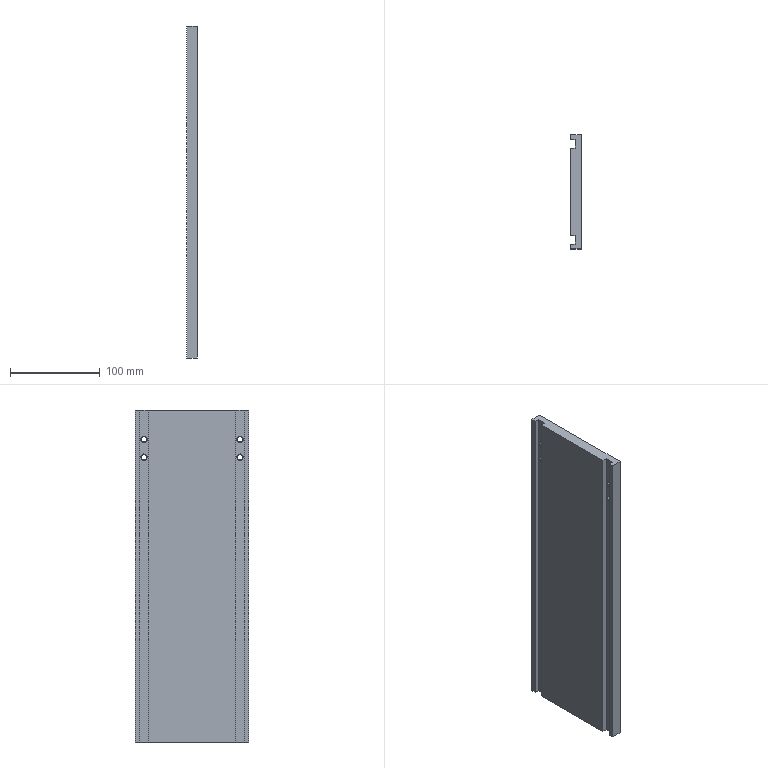Part | STEP file | Part7_5 | 1 solid | 44 faces | box 12 x 127 x 370 mm | volume 526068 mm3 | cone 22 | plane 14 | cylinder 8 | commonest cylinder face diameters 6 x8